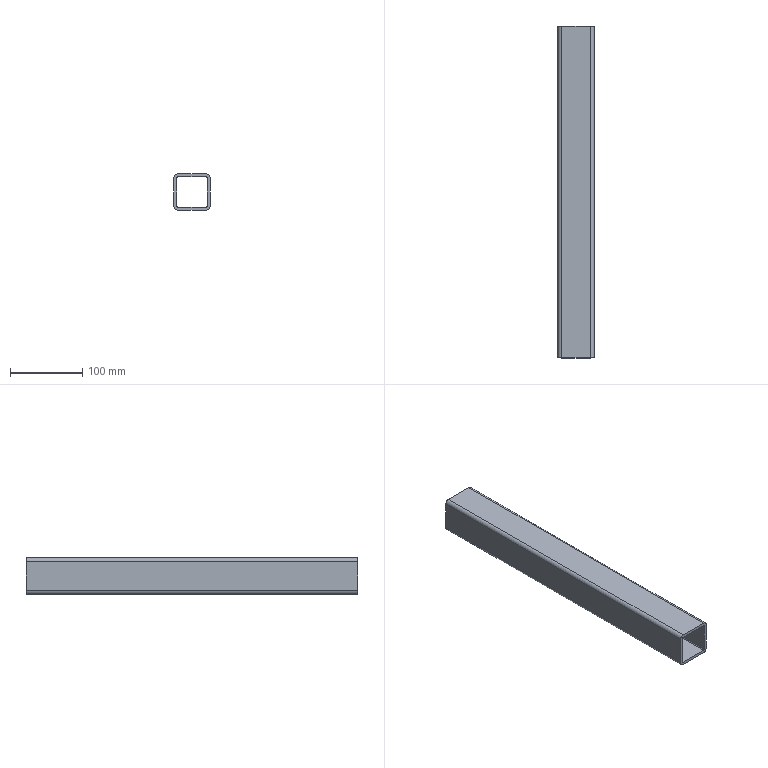Part | STEP file | 冲床-300配套压波_id726_x_t | 1 solid | 18 faces | box 50 x 460 x 50 mm | volume 329083 mm3 | plane 10 | cylinder 8 | commonest cylinder face diameters 2 x4 10 x4
STEP:
#1=CARTESIAN_POINT('',(1519.,230.,-775.));
#2=VERTEX_POINT('',#1);
#3=CARTESIAN_POINT('',(1519.,230.,-735.));
#4=VERTEX_POINT('',#3);
#5=CARTESIAN_POINT('',(1519.,230.,-980.));
#6=DIRECTION('',(0.,0.,1.));
#7=VECTOR('',#6,1.);
#8=LINE('',#5,#7);
#9=EDGE_CURVE('',#2,#4,#8,.T.);
#10=ORIENTED_EDGE('',*,*,#9,.F.);
#11=CARTESIAN_POINT('',(1520.,230.,-776.));
#12=VERTEX_POINT('',#11);
#13=CARTESIAN_POINT('',(1520.,230.,-775.));
#14=DIRECTION('',(0.,1.,0.));
#15=DIRECTION('',(1.,0.,0.));
#16=AXIS2_PLACEMENT_3D('',#13,#14,#15);
#17=CIRCLE('',#16,1.);
#18=EDGE_CURVE('',#12,#2,#17,.T.);
#19=ORIENTED_EDGE('',*,*,#18,.F.);
#20=CARTESIAN_POINT('',(1560.,230.,-776.));
#21=VERTEX_POINT('',#20);
#22=CARTESIAN_POINT('',(365.,230.,-776.));
#23=DIRECTION('',(-1.,0.,0.));
#24=VECTOR('',#23,1.);
#25=LINE('',#22,#24);
#26=EDGE_CURVE('',#21,#12,#25,.T.);
#27=ORIENTED_EDGE('',*,*,#26,.F.);
#28=CARTESIAN_POINT('',(1561.,230.,-775.));
#29=VERTEX_POINT('',#28);
#30=CARTESIAN_POINT('',(1560.,230.,-775.));
#31=DIRECTION('',(0.,1.,0.));
#32=DIRECTION('',(1.,0.,0.));
#33=AXIS2_PLACEMENT_3D('',#30,#31,#32);
#34=CIRCLE('',#33,1.);
#35=EDGE_CURVE('',#29,#21,#34,.T.);
#36=ORIENTED_EDGE('',*,*,#35,.F.);
#37=CARTESIAN_POINT('',(1561.,230.,-735.));
#38=VERTEX_POINT('',#37);
#39=CARTESIAN_POINT('',(1561.,230.,-980.));
#40=DIRECTION('',(0.,0.,-1.));
#41=VECTOR('',#40,1.);
#42=LINE('',#39,#41);
#43=EDGE_CURVE('',#38,#29,#42,.T.);
#44=ORIENTED_EDGE('',*,*,#43,.F.);
#45=CARTESIAN_POINT('',(1560.,230.,-734.));
#46=VERTEX_POINT('',#45);
#47=CARTESIAN_POINT('',(1560.,230.,-735.));
#48=DIRECTION('',(0.,1.,0.));
#49=DIRECTION('',(1.,0.,0.));
#50=AXIS2_PLACEMENT_3D('',#47,#48,#49);
#51=CIRCLE('',#50,1.);
#52=EDGE_CURVE('',#46,#38,#51,.T.);
#53=ORIENTED_EDGE('',*,*,#52,.F.);
#54=CARTESIAN_POINT('',(1520.,230.,-734.));
#55=VERTEX_POINT('',#54);
#56=CARTESIAN_POINT('',(365.,230.,-734.));
#57=DIRECTION('',(1.,0.,0.));
#58=VECTOR('',#57,1.);
#59=LINE('',#56,#58);
#60=EDGE_CURVE('',#55,#46,#59,.T.);
#61=ORIENTED_EDGE('',*,*,#60,.F.);
#62=CARTESIAN_POINT('',(1520.,230.,-735.));
#63=DIRECTION('',(0.,1.,0.));
#64=DIRECTION('',(1.,0.,0.));
#65=AXIS2_PLACEMENT_3D('',#62,#63,#64);
#66=CIRCLE('',#65,1.);
#67=EDGE_CURVE('',#4,#55,#66,.T.);
#68=ORIENTED_EDGE('',*,*,#67,.F.);
#69=EDGE_LOOP('',(#10,#19,#27,#36,#44,#53,#61,#68));
#70=FACE_BOUND('',#69,.T.);
#71=CARTESIAN_POINT('',(1515.,230.,-775.));
#72=VERTEX_POINT('',#71);
#73=CARTESIAN_POINT('',(1515.,230.,-735.));
#74=VERTEX_POINT('',#73);
#75=CARTESIAN_POINT('',(1515.,230.,-735.));
#76=DIRECTION('',(0.,0.,1.));
#77=VECTOR('',#76,1.);
#78=LINE('',#75,#77);
#79=EDGE_CURVE('',#72,#74,#78,.T.);
#80=ORIENTED_EDGE('',*,*,#79,.T.);
#81=CARTESIAN_POINT('',(1520.,230.,-730.));
#82=VERTEX_POINT('',#81);
#83=CARTESIAN_POINT('',(1520.,230.,-735.));
#84=DIRECTION('',(0.,1.,0.));
#85=DIRECTION('',(1.,0.,0.));
#86=AXIS2_PLACEMENT_3D('',#83,#84,#85);
#87=CIRCLE('',#86,5.);
#88=EDGE_CURVE('',#74,#82,#87,.T.);
#89=ORIENTED_EDGE('',*,*,#88,.T.);
#90=CARTESIAN_POINT('',(1560.,230.,-730.));
#91=VERTEX_POINT('',#90);
#92=CARTESIAN_POINT('',(1560.,230.,-730.));
#93=DIRECTION('',(1.,0.,0.));
#94=VECTOR('',#93,1.);
#95=LINE('',#92,#94);
#96=EDGE_CURVE('',#82,#91,#95,.T.);
#97=ORIENTED_EDGE('',*,*,#96,.T.);
#98=CARTESIAN_POINT('',(1565.,230.,-735.));
#99=VERTEX_POINT('',#98);
#100=CARTESIAN_POINT('',(1560.,230.,-735.));
#101=DIRECTION('',(0.,1.,0.));
#102=DIRECTION('',(1.,0.,0.));
#103=AXIS2_PLACEMENT_3D('',#100,#101,#102);
#104=CIRCLE('',#103,5.);
#105=EDGE_CURVE('',#91,#99,#104,.T.);
#106=ORIENTED_EDGE('',*,*,#105,.T.);
#107=CARTESIAN_POINT('',(1565.,230.,-775.));
#108=VERTEX_POINT('',#107);
#109=CARTESIAN_POINT('',(1565.,230.,-775.));
#110=DIRECTION('',(0.,0.,-1.));
#111=VECTOR('',#110,1.);
#112=LINE('',#109,#111);
#113=EDGE_CURVE('',#99,#108,#112,.T.);
#114=ORIENTED_EDGE('',*,*,#113,.T.);
#115=CARTESIAN_POINT('',(1560.,230.,-780.));
#116=VERTEX_POINT('',#115);
#117=CARTESIAN_POINT('',(1560.,230.,-775.));
#118=DIRECTION('',(0.,1.,0.));
#119=DIRECTION('',(1.,0.,0.));
#120=AXIS2_PLACEMENT_3D('',#117,#118,#119);
#121=CIRCLE('',#120,5.);
#122=EDGE_CURVE('',#108,#116,#121,.T.);
#123=ORIENTED_EDGE('',*,*,#122,.T.);
#124=CARTESIAN_POINT('',(1520.,230.,-780.));
#125=VERTEX_POINT('',#124);
#126=CARTESIAN_POINT('',(1520.,230.,-780.));
#127=DIRECTION('',(-1.,0.,0.));
#128=VECTOR('',#127,1.);
#129=LINE('',#126,#128);
#130=EDGE_CURVE('',#116,#125,#129,.T.);
#131=ORIENTED_EDGE('',*,*,#130,.T.);
#132=CARTESIAN_POINT('',(1520.,230.,-775.));
#133=DIRECTION('',(0.,1.,0.));
#134=DIRECTION('',(1.,0.,0.));
#135=AXIS2_PLACEMENT_3D('',#132,#133,#134);
#136=CIRCLE('',#135,5.);
#137=EDGE_CURVE('',#125,#72,#136,.T.);
#138=ORIENTED_EDGE('',*,*,#137,.T.);
#139=EDGE_LOOP('',(#80,#89,#97,#106,#114,#123,#131,#138));
#140=FACE_BOUND('',#139,.T.);
#141=CARTESIAN_POINT('',(365.,230.,-980.));
#142=DIRECTION('',(0.,1.,0.));
#143=DIRECTION('',(1.,0.,0.));
#144=AXIS2_PLACEMENT_3D('',#141,#142,#143);
#145=PLANE('',#144);
#146=ADVANCED_FACE('',(#70,#140),#145,.T.);
#147=CARTESIAN_POINT('',(1520.,-230.,-780.));
#148=VERTEX_POINT('',#147);
#149=CARTESIAN_POINT('',(1520.,-520.,-780.));
#150=DIRECTION('',(0.,-1.,0.));
#151=VECTOR('',#150,1.);
#152=LINE('',#149,#151);
#153=EDGE_CURVE('',#125,#148,#152,.T.);
#154=ORIENTED_EDGE('',*,*,#153,.T.);
#155=CARTESIAN_POINT('',(1515.,-230.,-775.));
#156=VERTEX_POINT('',#155);
#157=CARTESIAN_POINT('',(1520.,-230.,-775.));
#158=DIRECTION('',(0.,1.,0.));
#159=DIRECTION('',(1.,0.,0.));
#160=AXIS2_PLACEMENT_3D('',#157,#158,#159);
#161=CIRCLE('',#160,5.);
#162=EDGE_CURVE('',#148,#156,#161,.T.);
#163=ORIENTED_EDGE('',*,*,#162,.T.);
#164=CARTESIAN_POINT('',(1515.,-520.,-775.));
#165=DIRECTION('',(0.,-1.,0.));
#166=VECTOR('',#165,1.);
#167=LINE('',#164,#166);
#168=EDGE_CURVE('',#72,#156,#167,.T.);
#169=ORIENTED_EDGE('',*,*,#168,.F.);
#170=ORIENTED_EDGE('',*,*,#137,.F.);
#171=EDGE_LOOP('',(#154,#163,#169,#170));
#172=FACE_OUTER_BOUND('',#171,.T.);
#173=CARTESIAN_POINT('',(1520.,-520.,-775.));
#174=DIRECTION('',(0.,1.,0.));
#175=DIRECTION('',(1.,0.,0.));
#176=AXIS2_PLACEMENT_3D('',#173,#174,#175);
#177=CYLINDRICAL_SURFACE('',#176,5.);
#178=ADVANCED_FACE('',(#172),#177,.T.);
#179=CARTESIAN_POINT('',(1560.,-230.,-780.));
#180=VERTEX_POINT('',#179);
#181=CARTESIAN_POINT('',(1560.,-520.,-780.));
#182=DIRECTION('',(0.,-1.,0.));
#183=VECTOR('',#182,1.);
#184=LINE('',#181,#183);
#185=EDGE_CURVE('',#116,#180,#184,.T.);
#186=ORIENTED_EDGE('',*,*,#185,.T.);
#187=CARTESIAN_POINT('',(1520.,-230.,-780.));
#188=DIRECTION('',(-1.,0.,0.));
#189=VECTOR('',#188,1.);
#190=LINE('',#187,#189);
#191=EDGE_CURVE('',#180,#148,#190,.T.);
#192=ORIENTED_EDGE('',*,*,#191,.T.);
#193=ORIENTED_EDGE('',*,*,#153,.F.);
#194=ORIENTED_EDGE('',*,*,#130,.F.);
#195=EDGE_LOOP('',(#186,#192,#193,#194));
#196=FACE_OUTER_BOUND('',#195,.T.);
#197=CARTESIAN_POINT('',(1520.,-520.,-780.));
#198=DIRECTION('',(0.,0.,-1.));
#199=DIRECTION('',(1.,0.,0.));
#200=AXIS2_PLACEMENT_3D('',#197,#198,#199);
#201=PLANE('',#200);
#202=ADVANCED_FACE('',(#196),#201,.T.);
#203=CARTESIAN_POINT('',(1565.,-230.,-775.));
#204=VERTEX_POINT('',#203);
#205=CARTESIAN_POINT('',(1565.,-520.,-775.));
#206=DIRECTION('',(0.,-1.,0.));
#207=VECTOR('',#206,1.);
#208=LINE('',#205,#207);
#209=EDGE_CURVE('',#108,#204,#208,.T.);
#210=ORIENTED_EDGE('',*,*,#209,.T.);
#211=CARTESIAN_POINT('',(1560.,-230.,-775.));
#212=DIRECTION('',(0.,1.,0.));
#213=DIRECTION('',(1.,0.,0.));
#214=AXIS2_PLACEMENT_3D('',#211,#212,#213);
#215=CIRCLE('',#214,5.);
#216=EDGE_CURVE('',#204,#180,#215,.T.);
#217=ORIENTED_EDGE('',*,*,#216,.T.);
#218=ORIENTED_EDGE('',*,*,#185,.F.);
#219=ORIENTED_EDGE('',*,*,#122,.F.);
#220=EDGE_LOOP('',(#210,#217,#218,#219));
#221=FACE_OUTER_BOUND('',#220,.T.);
#222=CARTESIAN_POINT('',(1560.,-520.,-775.));
#223=DIRECTION('',(0.,1.,0.));
#224=DIRECTION('',(1.,0.,0.));
#225=AXIS2_PLACEMENT_3D('',#222,#223,#224);
#226=CYLINDRICAL_SURFACE('',#225,5.);
#227=ADVANCED_FACE('',(#221),#226,.T.);
#228=CARTESIAN_POINT('',(1565.,-230.,-735.));
#229=VERTEX_POINT('',#228);
#230=CARTESIAN_POINT('',(1565.,-520.,-735.));
#231=DIRECTION('',(0.,-1.,0.));
#232=VECTOR('',#231,1.);
#233=LINE('',#230,#232);
#234=EDGE_CURVE('',#99,#229,#233,.T.);
#235=ORIENTED_EDGE('',*,*,#234,.T.);
#236=CARTESIAN_POINT('',(1565.,-230.,-60.));
#237=DIRECTION('',(0.,0.,-1.));
#238=VECTOR('',#237,1.);
#239=LINE('',#236,#238);
#240=EDGE_CURVE('',#229,#204,#239,.T.);
#241=ORIENTED_EDGE('',*,*,#240,.T.);
#242=ORIENTED_EDGE('',*,*,#209,.F.);
#243=ORIENTED_EDGE('',*,*,#113,.F.);
#244=EDGE_LOOP('',(#235,#241,#242,#243));
#245=FACE_OUTER_BOUND('',#244,.T.);
#246=CARTESIAN_POINT('',(1565.,-520.,-775.));
#247=DIRECTION('',(1.,0.,0.));
#248=DIRECTION('',(0.,-1.,0.));
#249=AXIS2_PLACEMENT_3D('',#246,#247,#248);
#250=PLANE('',#249);
#251=ADVANCED_FACE('',(#245),#250,.T.);
#252=CARTESIAN_POINT('',(1560.,-230.,-730.));
#253=VERTEX_POINT('',#252);
#254=CARTESIAN_POINT('',(1560.,-520.,-730.));
#255=DIRECTION('',(0.,-1.,0.));
#256=VECTOR('',#255,1.);
#257=LINE('',#254,#256);
#258=EDGE_CURVE('',#91,#253,#257,.T.);
#259=ORIENTED_EDGE('',*,*,#258,.T.);
#260=CARTESIAN_POINT('',(1560.,-230.,-735.));
#261=DIRECTION('',(0.,1.,0.));
#262=DIRECTION('',(1.,0.,0.));
#263=AXIS2_PLACEMENT_3D('',#260,#261,#262);
#264=CIRCLE('',#263,5.);
#265=EDGE_CURVE('',#253,#229,#264,.T.);
#266=ORIENTED_EDGE('',*,*,#265,.T.);
#267=ORIENTED_EDGE('',*,*,#234,.F.);
#268=ORIENTED_EDGE('',*,*,#105,.F.);
#269=EDGE_LOOP('',(#259,#266,#267,#268));
#270=FACE_OUTER_BOUND('',#269,.T.);
#271=CARTESIAN_POINT('',(1560.,-520.,-735.));
#272=DIRECTION('',(0.,1.,0.));
#273=DIRECTION('',(1.,0.,0.));
#274=AXIS2_PLACEMENT_3D('',#271,#272,#273);
#275=CYLINDRICAL_SURFACE('',#274,5.);
#276=ADVANCED_FACE('',(#270),#275,.T.);
#277=CARTESIAN_POINT('',(1519.,-230.,-735.));
#278=VERTEX_POINT('',#277);
#279=CARTESIAN_POINT('',(1520.,-230.,-734.));
#280=VERTEX_POINT('',#279);
#281=CARTESIAN_POINT('',(1520.,-230.,-735.));
#282=DIRECTION('',(0.,1.,0.));
#283=DIRECTION('',(1.,0.,0.));
#284=AXIS2_PLACEMENT_3D('',#281,#282,#283);
#285=CIRCLE('',#284,1.);
#286=EDGE_CURVE('',#278,#280,#285,.T.);
#287=ORIENTED_EDGE('',*,*,#286,.T.);
#288=CARTESIAN_POINT('',(1560.,-230.,-734.));
#289=VERTEX_POINT('',#288);
#290=CARTESIAN_POINT('',(1520.,-230.,-734.));
#291=DIRECTION('',(1.,0.,0.));
#292=VECTOR('',#291,1.);
#293=LINE('',#290,#292);
#294=EDGE_CURVE('',#280,#289,#293,.T.);
#295=ORIENTED_EDGE('',*,*,#294,.T.);
#296=CARTESIAN_POINT('',(1561.,-230.,-735.));
#297=VERTEX_POINT('',#296);
#298=CARTESIAN_POINT('',(1560.,-230.,-735.));
#299=DIRECTION('',(0.,1.,0.));
#300=DIRECTION('',(1.,0.,0.));
#301=AXIS2_PLACEMENT_3D('',#298,#299,#300);
#302=CIRCLE('',#301,1.);
#303=EDGE_CURVE('',#289,#297,#302,.T.);
#304=ORIENTED_EDGE('',*,*,#303,.T.);
#305=CARTESIAN_POINT('',(1561.,-230.,-775.));
#306=VERTEX_POINT('',#305);
#307=CARTESIAN_POINT('',(1561.,-230.,-60.));
#308=DIRECTION('',(0.,0.,-1.));
#309=VECTOR('',#308,1.);
#310=LINE('',#307,#309);
#311=EDGE_CURVE('',#297,#306,#310,.T.);
#312=ORIENTED_EDGE('',*,*,#311,.T.);
#313=CARTESIAN_POINT('',(1560.,-230.,-776.));
#314=VERTEX_POINT('',#313);
#315=CARTESIAN_POINT('',(1560.,-230.,-775.));
#316=DIRECTION('',(0.,1.,0.));
#317=DIRECTION('',(1.,0.,0.));
#318=AXIS2_PLACEMENT_3D('',#315,#316,#317);
#319=CIRCLE('',#318,1.);
#320=EDGE_CURVE('',#306,#314,#319,.T.);
#321=ORIENTED_EDGE('',*,*,#320,.T.);
#322=CARTESIAN_POINT('',(1520.,-230.,-776.));
#323=VERTEX_POINT('',#322);
#324=CARTESIAN_POINT('',(1520.,-230.,-776.));
#325=DIRECTION('',(-1.,0.,0.));
#326=VECTOR('',#325,1.);
#327=LINE('',#324,#326);
#328=EDGE_CURVE('',#314,#323,#327,.T.);
#329=ORIENTED_EDGE('',*,*,#328,.T.);
#330=CARTESIAN_POINT('',(1519.,-230.,-775.));
#331=VERTEX_POINT('',#330);
#332=CARTESIAN_POINT('',(1520.,-230.,-775.));
#333=DIRECTION('',(0.,1.,0.));
#334=DIRECTION('',(1.,0.,0.));
#335=AXIS2_PLACEMENT_3D('',#332,#333,#334);
#336=CIRCLE('',#335,1.);
#337=EDGE_CURVE('',#323,#331,#336,.T.);
#338=ORIENTED_EDGE('',*,*,#337,.T.);
#339=CARTESIAN_POINT('',(1519.,-230.,-60.));
#340=DIRECTION('',(0.,0.,1.));
#341=VECTOR('',#340,1.);
#342=LINE('',#339,#341);
#343=EDGE_CURVE('',#331,#278,#342,.T.);
#344=ORIENTED_EDGE('',*,*,#343,.T.);
#345=EDGE_LOOP('',(#287,#295,#304,#312,#321,#329,#338,#344));
#346=FACE_BOUND('',#345,.T.);
#347=CARTESIAN_POINT('',(1515.,-230.,-735.));
#348=VERTEX_POINT('',#347);
#349=CARTESIAN_POINT('',(1515.,-230.,-60.));
#350=DIRECTION('',(0.,0.,1.));
#351=VECTOR('',#350,1.);
#352=LINE('',#349,#351);
#353=EDGE_CURVE('',#156,#348,#352,.T.);
#354=ORIENTED_EDGE('',*,*,#353,.F.);
#355=ORIENTED_EDGE('',*,*,#162,.F.);
#356=ORIENTED_EDGE('',*,*,#191,.F.);
#357=ORIENTED_EDGE('',*,*,#216,.F.);
#358=ORIENTED_EDGE('',*,*,#240,.F.);
#359=ORIENTED_EDGE('',*,*,#265,.F.);
#360=CARTESIAN_POINT('',(1520.,-230.,-730.));
#361=VERTEX_POINT('',#360);
#362=CARTESIAN_POINT('',(1520.,-230.,-730.));
#363=DIRECTION('',(1.,0.,0.));
#364=VECTOR('',#363,1.);
#365=LINE('',#362,#364);
#366=EDGE_CURVE('',#361,#253,#365,.T.);
#367=ORIENTED_EDGE('',*,*,#366,.F.);
#368=CARTESIAN_POINT('',(1520.,-230.,-735.));
#369=DIRECTION('',(0.,1.,0.));
#370=DIRECTION('',(1.,0.,0.));
#371=AXIS2_PLACEMENT_3D('',#368,#369,#370);
#372=CIRCLE('',#371,5.);
#373=EDGE_CURVE('',#348,#361,#372,.T.);
#374=ORIENTED_EDGE('',*,*,#373,.F.);
#375=EDGE_LOOP('',(#354,#355,#356,#357,#358,#359,#367,#374));
#376=FACE_BOUND('',#375,.T.);
#377=CARTESIAN_POINT('',(1520.,-230.,-60.));
#378=DIRECTION('',(0.,1.,0.));
#379=DIRECTION('',(1.,0.,0.));
#380=AXIS2_PLACEMENT_3D('',#377,#378,#379);
#381=PLANE('',#380);
#382=ADVANCED_FACE('',(#346,#376),#381,.F.);
#383=CARTESIAN_POINT('',(1520.,-520.,-730.));
#384=DIRECTION('',(0.,-1.,0.));
#385=VECTOR('',#384,1.);
#386=LINE('',#383,#385);
#387=EDGE_CURVE('',#82,#361,#386,.T.);
#388=ORIENTED_EDGE('',*,*,#387,.T.);
#389=ORIENTED_EDGE('',*,*,#366,.T.);
#390=ORIENTED_EDGE('',*,*,#258,.F.);
#391=ORIENTED_EDGE('',*,*,#96,.F.);
#392=EDGE_LOOP('',(#388,#389,#390,#391));
#393=FACE_OUTER_BOUND('',#392,.T.);
#394=CARTESIAN_POINT('',(1560.,-520.,-730.));
#395=DIRECTION('',(0.,0.,1.));
#396=DIRECTION('',(-1.,0.,0.));
#397=AXIS2_PLACEMENT_3D('',#394,#395,#396);
#398=PLANE('',#397);
#399=ADVANCED_FACE('',(#393),#398,.T.);
#400=ORIENTED_EDGE('',*,*,#168,.T.);
#401=ORIENTED_EDGE('',*,*,#353,.T.);
#402=CARTESIAN_POINT('',(1515.,-520.,-735.));
#403=DIRECTION('',(0.,-1.,0.));
#404=VECTOR('',#403,1.);
#405=LINE('',#402,#404);
#406=EDGE_CURVE('',#74,#348,#405,.T.);
#407=ORIENTED_EDGE('',*,*,#406,.F.);
#408=ORIENTED_EDGE('',*,*,#79,.F.);
#409=EDGE_LOOP('',(#400,#401,#407,#408));
#410=FACE_OUTER_BOUND('',#409,.T.);
#411=CARTESIAN_POINT('',(1515.,-520.,-735.));
#412=DIRECTION('',(-1.,0.,0.));
#413=DIRECTION('',(0.,1.,0.));
#414=AXIS2_PLACEMENT_3D('',#411,#412,#413);
#415=PLANE('',#414);
#416=ADVANCED_FACE('',(#410),#415,.T.);
#417=ORIENTED_EDGE('',*,*,#406,.T.);
#418=ORIENTED_EDGE('',*,*,#373,.T.);
#419=ORIENTED_EDGE('',*,*,#387,.F.);
#420=ORIENTED_EDGE('',*,*,#88,.F.);
#421=EDGE_LOOP('',(#417,#418,#419,#420));
#422=FACE_OUTER_BOUND('',#421,.T.);
#423=CARTESIAN_POINT('',(1520.,-520.,-735.));
#424=DIRECTION('',(0.,1.,0.));
#425=DIRECTION('',(1.,0.,0.));
#426=AXIS2_PLACEMENT_3D('',#423,#424,#425);
#427=CYLINDRICAL_SURFACE('',#426,5.);
#428=ADVANCED_FACE('',(#422),#427,.T.);
#429=CARTESIAN_POINT('',(1520.,-520.,-776.));
#430=DIRECTION('',(0.,-1.,0.));
#431=VECTOR('',#430,1.);
#432=LINE('',#429,#431);
#433=EDGE_CURVE('',#12,#323,#432,.T.);
#434=ORIENTED_EDGE('',*,*,#433,.F.);
#435=ORIENTED_EDGE('',*,*,#18,.T.);
#436=CARTESIAN_POINT('',(1519.,-520.,-775.));
#437=DIRECTION('',(0.,-1.,0.));
#438=VECTOR('',#437,1.);
#439=LINE('',#436,#438);
#440=EDGE_CURVE('',#2,#331,#439,.T.);
#441=ORIENTED_EDGE('',*,*,#440,.T.);
#442=ORIENTED_EDGE('',*,*,#337,.F.);
#443=EDGE_LOOP('',(#434,#435,#441,#442));
#444=FACE_OUTER_BOUND('',#443,.T.);
#445=CARTESIAN_POINT('',(1520.,-520.,-775.));
#446=DIRECTION('',(0.,1.,0.));
#447=DIRECTION('',(1.,0.,0.));
#448=AXIS2_PLACEMENT_3D('',#445,#446,#447);
#449=CYLINDRICAL_SURFACE('',#448,1.);
#450=ADVANCED_FACE('',(#444),#449,.F.);
#451=CARTESIAN_POINT('',(1560.,-520.,-776.));
#452=DIRECTION('',(0.,-1.,0.));
#453=VECTOR('',#452,1.);
#454=LINE('',#451,#453);
#455=EDGE_CURVE('',#21,#314,#454,.T.);
#456=ORIENTED_EDGE('',*,*,#455,.F.);
#457=ORIENTED_EDGE('',*,*,#26,.T.);
#458=ORIENTED_EDGE('',*,*,#433,.T.);
#459=ORIENTED_EDGE('',*,*,#328,.F.);
#460=EDGE_LOOP('',(#456,#457,#458,#459));
#461=FACE_OUTER_BOUND('',#460,.T.);
#462=CARTESIAN_POINT('',(1520.,-520.,-776.));
#463=DIRECTION('',(0.,0.,-1.));
#464=DIRECTION('',(1.,0.,0.));
#465=AXIS2_PLACEMENT_3D('',#462,#463,#464);
#466=PLANE('',#465);
#467=ADVANCED_FACE('',(#461),#466,.F.);
#468=CARTESIAN_POINT('',(1561.,-520.,-775.));
#469=DIRECTION('',(0.,-1.,0.));
#470=VECTOR('',#469,1.);
#471=LINE('',#468,#470);
#472=EDGE_CURVE('',#29,#306,#471,.T.);
#473=ORIENTED_EDGE('',*,*,#472,.F.);
#474=ORIENTED_EDGE('',*,*,#35,.T.);
#475=ORIENTED_EDGE('',*,*,#455,.T.);
#476=ORIENTED_EDGE('',*,*,#320,.F.);
#477=EDGE_LOOP('',(#473,#474,#475,#476));
#478=FACE_OUTER_BOUND('',#477,.T.);
#479=CARTESIAN_POINT('',(1560.,-520.,-775.));
#480=DIRECTION('',(0.,1.,0.));
#481=DIRECTION('',(1.,0.,0.));
#482=AXIS2_PLACEMENT_3D('',#479,#480,#481);
#483=CYLINDRICAL_SURFACE('',#482,1.);
#484=ADVANCED_FACE('',(#478),#483,.F.);
#485=CARTESIAN_POINT('',(1561.,-520.,-735.));
#486=DIRECTION('',(0.,-1.,0.));
#487=VECTOR('',#486,1.);
#488=LINE('',#485,#487);
#489=EDGE_CURVE('',#38,#297,#488,.T.);
#490=ORIENTED_EDGE('',*,*,#489,.F.);
#491=ORIENTED_EDGE('',*,*,#43,.T.);
#492=ORIENTED_EDGE('',*,*,#472,.T.);
#493=ORIENTED_EDGE('',*,*,#311,.F.);
#494=EDGE_LOOP('',(#490,#491,#492,#493));
#495=FACE_OUTER_BOUND('',#494,.T.);
#496=CARTESIAN_POINT('',(1561.,-520.,-775.));
#497=DIRECTION('',(1.,0.,0.));
#498=DIRECTION('',(0.,-1.,0.));
#499=AXIS2_PLACEMENT_3D('',#496,#497,#498);
#500=PLANE('',#499);
#501=ADVANCED_FACE('',(#495),#500,.F.);
#502=CARTESIAN_POINT('',(1560.,-520.,-734.));
#503=DIRECTION('',(0.,-1.,0.));
#504=VECTOR('',#503,1.);
#505=LINE('',#502,#504);
#506=EDGE_CURVE('',#46,#289,#505,.T.);
#507=ORIENTED_EDGE('',*,*,#506,.F.);
#508=ORIENTED_EDGE('',*,*,#52,.T.);
#509=ORIENTED_EDGE('',*,*,#489,.T.);
#510=ORIENTED_EDGE('',*,*,#303,.F.);
#511=EDGE_LOOP('',(#507,#508,#509,#510));
#512=FACE_OUTER_BOUND('',#511,.T.);
#513=CARTESIAN_POINT('',(1560.,-520.,-735.));
#514=DIRECTION('',(0.,1.,0.));
#515=DIRECTION('',(1.,0.,0.));
#516=AXIS2_PLACEMENT_3D('',#513,#514,#515);
#517=CYLINDRICAL_SURFACE('',#516,1.);
#518=ADVANCED_FACE('',(#512),#517,.F.);
#519=CARTESIAN_POINT('',(1520.,-520.,-734.));
#520=DIRECTION('',(0.,-1.,0.));
#521=VECTOR('',#520,1.);
#522=LINE('',#519,#521);
#523=EDGE_CURVE('',#55,#280,#522,.T.);
#524=ORIENTED_EDGE('',*,*,#523,.F.);
#525=ORIENTED_EDGE('',*,*,#60,.T.);
#526=ORIENTED_EDGE('',*,*,#506,.T.);
#527=ORIENTED_EDGE('',*,*,#294,.F.);
#528=EDGE_LOOP('',(#524,#525,#526,#527));
#529=FACE_OUTER_BOUND('',#528,.T.);
#530=CARTESIAN_POINT('',(1560.,-520.,-734.));
#531=DIRECTION('',(0.,0.,1.));
#532=DIRECTION('',(-1.,0.,0.));
#533=AXIS2_PLACEMENT_3D('',#530,#531,#532);
#534=PLANE('',#533);
#535=ADVANCED_FACE('',(#529),#534,.F.);
#536=ORIENTED_EDGE('',*,*,#440,.F.);
#537=ORIENTED_EDGE('',*,*,#9,.T.);
#538=CARTESIAN_POINT('',(1519.,-520.,-735.));
#539=DIRECTION('',(0.,-1.,0.));
#540=VECTOR('',#539,1.);
#541=LINE('',#538,#540);
#542=EDGE_CURVE('',#4,#278,#541,.T.);
#543=ORIENTED_EDGE('',*,*,#542,.T.);
#544=ORIENTED_EDGE('',*,*,#343,.F.);
#545=EDGE_LOOP('',(#536,#537,#543,#544));
#546=FACE_OUTER_BOUND('',#545,.T.);
#547=CARTESIAN_POINT('',(1519.,-520.,-735.));
#548=DIRECTION('',(-1.,0.,0.));
#549=DIRECTION('',(0.,1.,0.));
#550=AXIS2_PLACEMENT_3D('',#547,#548,#549);
#551=PLANE('',#550);
#552=ADVANCED_FACE('',(#546),#551,.F.);
#553=ORIENTED_EDGE('',*,*,#542,.F.);
#554=ORIENTED_EDGE('',*,*,#67,.T.);
#555=ORIENTED_EDGE('',*,*,#523,.T.);
#556=ORIENTED_EDGE('',*,*,#286,.F.);
#557=EDGE_LOOP('',(#553,#554,#555,#556));
#558=FACE_OUTER_BOUND('',#557,.T.);
#559=CARTESIAN_POINT('',(1520.,-520.,-735.));
#560=DIRECTION('',(0.,1.,0.));
#561=DIRECTION('',(1.,0.,0.));
#562=AXIS2_PLACEMENT_3D('',#559,#560,#561);
#563=CYLINDRICAL_SURFACE('',#562,1.);
#564=ADVANCED_FACE('',(#558),#563,.F.);
#565=CLOSED_SHELL('',(#146,#178,#202,#227,#251,#276,#382,#399,#416,#428,#450,#467,#484,#501,#518,#535,#552,#564));
#566=MANIFOLD_SOLID_BREP('',#565);
#567=(LENGTH_UNIT()NAMED_UNIT(*)SI_UNIT(.MILLI.,.METRE.));
#568=UNCERTAINTY_MEASURE_WITH_UNIT(LENGTH_MEASURE(0.00002),#567,'','');
#569=(NAMED_UNIT(*)PLANE_ANGLE_UNIT()SI_UNIT($,.RADIAN.));
#570=PLANE_ANGLE_MEASURE_WITH_UNIT(PLANE_ANGLE_MEASURE(0.01745),#569);
#571=DIMENSIONAL_EXPONENTS(0.,0.,0.,0.,0.,0.,0.);
#572=(CONVERSION_BASED_UNIT('DEGREE',#570)NAMED_UNIT(#571)PLANE_ANGLE_UNIT());
#573=(NAMED_UNIT(*)SI_UNIT($,.STERADIAN.)SOLID_ANGLE_UNIT());
#574=(GEOMETRIC_REPRESENTATION_CONTEXT(3)GLOBAL_UNCERTAINTY_ASSIGNED_CONTEXT((#568))GLOBAL_UNIT_ASSIGNED_CONTEXT((#567,#572,#573))REPRESENTATION_CONTEXT('',''));
#575=ADVANCED_BREP_SHAPE_REPRESENTATION('',(#566),#574);